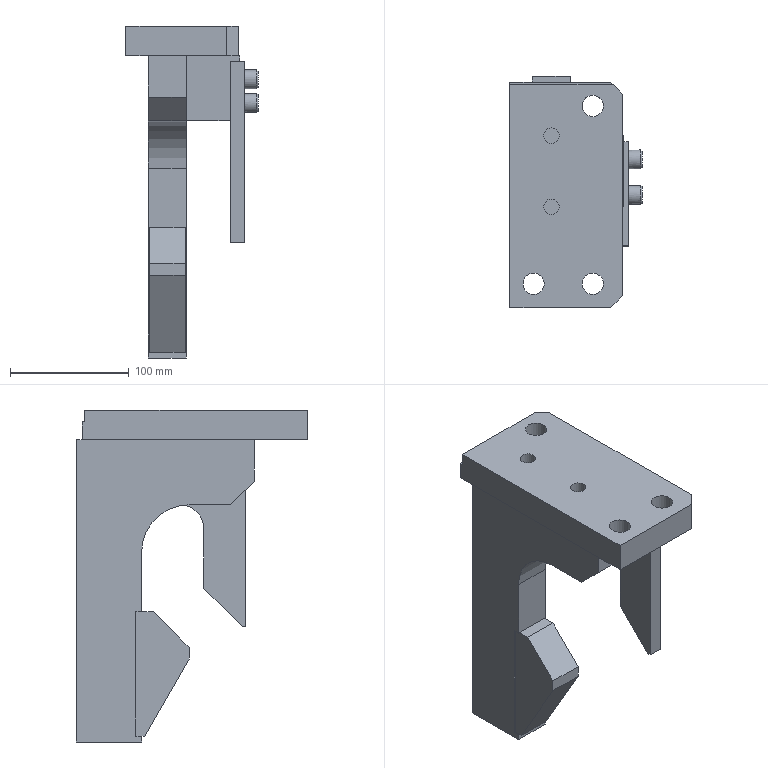Part | NX | features solid 2 | 1 solid | 74 faces | box 111.5 x 195 x 280 mm | volume 1336544 mm3 | plane 58 | cylinder 12 | cone 4 | commonest cylinder face diameters 18 x3 26 x3 13 x2 16 x2 40 x1 80 x1